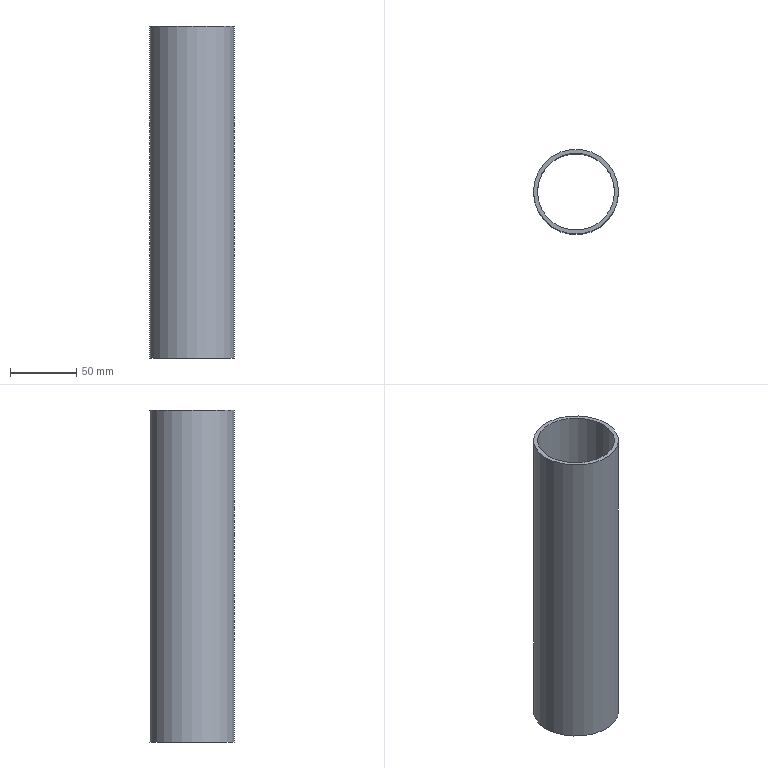Part | STEP file | JBJ-P-1000-01 | 1 solid | 4 faces | box 64 x 64 x 250 mm | volume 143728 mm3 | plane 2 | cylinder 2 | commonest cylinder face diameters 58 x1 64 x1
STEP:
#1=CARTESIAN_POINT('',(32.,0.,250.));
#2=VERTEX_POINT('',#1);
#3=CARTESIAN_POINT('',(0.,0.,250.));
#4=DIRECTION('',(0.,0.,1.));
#5=DIRECTION('',(1.,0.,0.));
#6=AXIS2_PLACEMENT_3D('',#3,#4,#5);
#7=CIRCLE('',#6,32.);
#8=EDGE_CURVE('',#2,#2,#7,.T.);
#9=ORIENTED_EDGE('',*,*,#8,.T.);
#10=EDGE_LOOP('',(#9));
#11=FACE_OUTER_BOUND('',#10,.T.);
#12=CARTESIAN_POINT('',(29.,0.,250.));
#13=VERTEX_POINT('',#12);
#14=CARTESIAN_POINT('',(0.,0.,250.));
#15=DIRECTION('',(0.,0.,1.));
#16=DIRECTION('',(1.,0.,0.));
#17=AXIS2_PLACEMENT_3D('',#14,#15,#16);
#18=CIRCLE('',#17,29.);
#19=EDGE_CURVE('',#13,#13,#18,.T.);
#20=ORIENTED_EDGE('',*,*,#19,.F.);
#21=EDGE_LOOP('',(#20));
#22=FACE_BOUND('',#21,.T.);
#23=CARTESIAN_POINT('',(0.,0.,250.));
#24=DIRECTION('',(0.,0.,1.));
#25=DIRECTION('',(1.,0.,0.));
#26=AXIS2_PLACEMENT_3D('',#23,#24,#25);
#27=PLANE('',#26);
#28=ADVANCED_FACE('',(#11,#22),#27,.T.);
#29=CARTESIAN_POINT('',(32.,0.,0.));
#30=VERTEX_POINT('',#29);
#31=CARTESIAN_POINT('',(0.,0.,0.));
#32=DIRECTION('',(0.,0.,1.));
#33=DIRECTION('',(1.,0.,0.));
#34=AXIS2_PLACEMENT_3D('',#31,#32,#33);
#35=CIRCLE('',#34,32.);
#36=EDGE_CURVE('',#30,#30,#35,.T.);
#37=ORIENTED_EDGE('',*,*,#36,.F.);
#38=EDGE_LOOP('',(#37));
#39=FACE_OUTER_BOUND('',#38,.T.);
#40=CARTESIAN_POINT('',(29.,0.,0.));
#41=VERTEX_POINT('',#40);
#42=CARTESIAN_POINT('',(0.,0.,0.));
#43=DIRECTION('',(0.,0.,1.));
#44=DIRECTION('',(1.,0.,0.));
#45=AXIS2_PLACEMENT_3D('',#42,#43,#44);
#46=CIRCLE('',#45,29.);
#47=EDGE_CURVE('',#41,#41,#46,.T.);
#48=ORIENTED_EDGE('',*,*,#47,.T.);
#49=EDGE_LOOP('',(#48));
#50=FACE_BOUND('',#49,.T.);
#51=CARTESIAN_POINT('',(0.,0.,0.));
#52=DIRECTION('',(0.,0.,1.));
#53=DIRECTION('',(1.,0.,0.));
#54=AXIS2_PLACEMENT_3D('',#51,#52,#53);
#55=PLANE('',#54);
#56=ADVANCED_FACE('',(#39,#50),#55,.F.);
#57=ORIENTED_EDGE('',*,*,#8,.F.);
#58=EDGE_LOOP('',(#57));
#59=FACE_OUTER_BOUND('',#58,.T.);
#60=ORIENTED_EDGE('',*,*,#36,.T.);
#61=EDGE_LOOP('',(#60));
#62=FACE_OUTER_BOUND('',#61,.T.);
#63=CARTESIAN_POINT('',(0.,0.,250.));
#64=DIRECTION('',(0.,0.,-1.));
#65=DIRECTION('',(-1.,0.,0.));
#66=AXIS2_PLACEMENT_3D('',#63,#64,#65);
#67=CYLINDRICAL_SURFACE('',#66,32.);
#68=ADVANCED_FACE('',(#59,#62),#67,.T.);
#69=ORIENTED_EDGE('',*,*,#19,.T.);
#70=EDGE_LOOP('',(#69));
#71=FACE_OUTER_BOUND('',#70,.T.);
#72=ORIENTED_EDGE('',*,*,#47,.F.);
#73=EDGE_LOOP('',(#72));
#74=FACE_OUTER_BOUND('',#73,.T.);
#75=CARTESIAN_POINT('',(0.,0.,250.));
#76=DIRECTION('',(0.,0.,-1.));
#77=DIRECTION('',(-1.,0.,0.));
#78=AXIS2_PLACEMENT_3D('',#75,#76,#77);
#79=CYLINDRICAL_SURFACE('',#78,29.);
#80=ADVANCED_FACE('',(#71,#74),#79,.F.);
#81=CLOSED_SHELL('',(#28,#56,#68,#80));
#82=MANIFOLD_SOLID_BREP('',#81);
#83=CARTESIAN_POINT('',(0.,0.,0.));
#84=DIRECTION('',(0.,0.,1.));
#85=DIRECTION('',(1.,0.,0.));
#86=AXIS2_PLACEMENT_3D('',#83,#84,#85);
#87=(LENGTH_UNIT()NAMED_UNIT(*)SI_UNIT(.MILLI.,.METRE.));
#88=UNCERTAINTY_MEASURE_WITH_UNIT(LENGTH_MEASURE(0.00001),#87,'','');
#89=(NAMED_UNIT(*)PLANE_ANGLE_UNIT()SI_UNIT($,.RADIAN.));
#90=(NAMED_UNIT(*)SI_UNIT($,.STERADIAN.)SOLID_ANGLE_UNIT());
#91=(GEOMETRIC_REPRESENTATION_CONTEXT(3)GLOBAL_UNCERTAINTY_ASSIGNED_CONTEXT((#88))GLOBAL_UNIT_ASSIGNED_CONTEXT((#87,#89,#90))REPRESENTATION_CONTEXT('',''));
#92=ADVANCED_BREP_SHAPE_REPRESENTATION('',(#82,#86),#91);